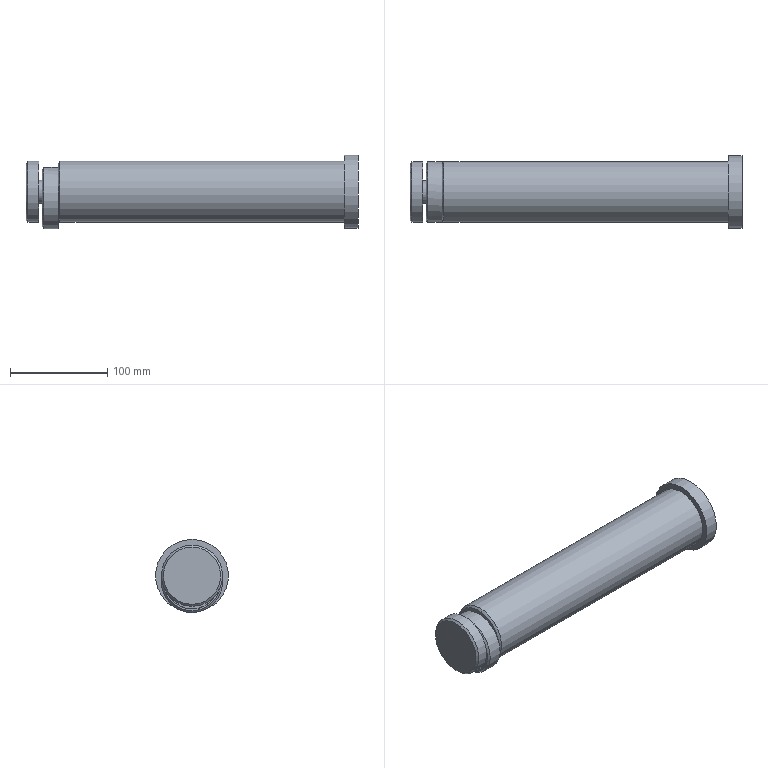Part | NX | features solid 2 | 1 solid | 17 faces | box 342 x 75 x 75.5 mm | volume 1041620 mm3 | plane 8 | cylinder 6 | cone 3 | commonest cylinder face diameters 63 x3 23.625 x1 55.5 x1 75 x1
STEP:
#1=CARTESIAN_POINT('',(940.,-806.145,-408.865));
#2=VERTEX_POINT('',#1);
#3=CARTESIAN_POINT('',(940.,-863.855,-408.865));
#4=VERTEX_POINT('',#3);
#5=CARTESIAN_POINT('',(940.,-835.,-421.5));
#6=DIRECTION('',(1.,0.,0.));
#7=DIRECTION('',(0.,0.,-1.));
#8=AXIS2_PLACEMENT_3D('',#5,#6,#7);
#9=CIRCLE('',#8,31.5);
#10=EDGE_CURVE('',#2,#4,#9,.T.);
#11=ORIENTED_EDGE('',*,*,#10,.T.);
#12=CARTESIAN_POINT('',(940.,-835.,-415.));
#13=DIRECTION('',(1.,0.,0.));
#14=DIRECTION('',(0.,0.,-1.));
#15=AXIS2_PLACEMENT_3D('',#12,#13,#14);
#16=CIRCLE('',#15,29.5);
#17=EDGE_CURVE('',#2,#4,#16,.T.);
#18=ORIENTED_EDGE('',*,*,#17,.F.);
#19=EDGE_LOOP('',(#11,#18));
#20=FACE_BOUND('',#19,.T.);
#21=CARTESIAN_POINT('',(940.,-835.,-415.));
#22=DIRECTION('',(-1.,0.,0.));
#23=DIRECTION('',(0.,0.,1.));
#24=AXIS2_PLACEMENT_3D('',#21,#22,#23);
#25=PLANE('',#24);
#26=ADVANCED_FACE('',(#20),#25,.T.);
#27=CARTESIAN_POINT('',(942.,-835.,-446.5));
#28=VERTEX_POINT('',#27);
#29=CARTESIAN_POINT('',(942.,-835.,-415.));
#30=DIRECTION('',(-1.,0.,0.));
#31=DIRECTION('',(0.,0.,-1.));
#32=AXIS2_PLACEMENT_3D('',#29,#30,#31);
#33=CIRCLE('',#32,31.5);
#34=EDGE_CURVE('',#28,#28,#33,.T.);
#35=ORIENTED_EDGE('',*,*,#34,.F.);
#36=EDGE_LOOP('',(#35));
#37=FACE_BOUND('',#36,.T.);
#38=CARTESIAN_POINT('',(1235.,-835.,-446.5));
#39=VERTEX_POINT('',#38);
#40=CARTESIAN_POINT('',(1235.,-835.,-415.));
#41=DIRECTION('',(-1.,0.,0.));
#42=DIRECTION('',(0.,0.,-1.));
#43=AXIS2_PLACEMENT_3D('',#40,#41,#42);
#44=CIRCLE('',#43,31.5);
#45=EDGE_CURVE('',#39,#39,#44,.T.);
#46=ORIENTED_EDGE('',*,*,#45,.T.);
#47=EDGE_LOOP('',(#46));
#48=FACE_BOUND('',#47,.T.);
#49=CARTESIAN_POINT('',(1235.,-835.,-415.));
#50=DIRECTION('',(-1.,0.,0.));
#51=DIRECTION('',(0.,0.,1.));
#52=AXIS2_PLACEMENT_3D('',#49,#50,#51);
#53=CYLINDRICAL_SURFACE('',#52,31.5);
#54=ADVANCED_FACE('',(#37,#48),#53,.T.);
#55=CARTESIAN_POINT('',(1249.,-835.,-377.5));
#56=VERTEX_POINT('',#55);
#57=CARTESIAN_POINT('',(1249.,-835.,-415.));
#58=DIRECTION('',(-1.,0.,0.));
#59=DIRECTION('',(0.,0.,1.));
#60=AXIS2_PLACEMENT_3D('',#57,#58,#59);
#61=CIRCLE('',#60,37.5);
#62=EDGE_CURVE('',#56,#56,#61,.T.);
#63=ORIENTED_EDGE('',*,*,#62,.F.);
#64=EDGE_LOOP('',(#63));
#65=FACE_BOUND('',#64,.T.);
#66=CARTESIAN_POINT('',(1249.,-835.,-415.));
#67=DIRECTION('',(1.,0.,0.));
#68=DIRECTION('',(0.,0.,-1.));
#69=AXIS2_PLACEMENT_3D('',#66,#67,#68);
#70=PLANE('',#69);
#71=ADVANCED_FACE('',(#65),#70,.T.);
#72=ORIENTED_EDGE('',*,*,#45,.F.);
#73=EDGE_LOOP('',(#72));
#74=FACE_BOUND('',#73,.T.);
#75=CARTESIAN_POINT('',(1235.,-835.,-377.5));
#76=VERTEX_POINT('',#75);
#77=CARTESIAN_POINT('',(1235.,-835.,-415.));
#78=DIRECTION('',(-1.,0.,0.));
#79=DIRECTION('',(0.,0.,1.));
#80=AXIS2_PLACEMENT_3D('',#77,#78,#79);
#81=CIRCLE('',#80,37.5);
#82=EDGE_CURVE('',#76,#76,#81,.T.);
#83=ORIENTED_EDGE('',*,*,#82,.T.);
#84=EDGE_LOOP('',(#83));
#85=FACE_BOUND('',#84,.T.);
#86=CARTESIAN_POINT('',(1235.,-835.,-415.));
#87=DIRECTION('',(-1.,0.,0.));
#88=DIRECTION('',(0.,0.,1.));
#89=AXIS2_PLACEMENT_3D('',#86,#87,#88);
#90=PLANE('',#89);
#91=ADVANCED_FACE('',(#74,#85),#90,.T.);
#92=ORIENTED_EDGE('',*,*,#62,.T.);
#93=EDGE_LOOP('',(#92));
#94=FACE_BOUND('',#93,.T.);
#95=ORIENTED_EDGE('',*,*,#82,.F.);
#96=EDGE_LOOP('',(#95));
#97=FACE_BOUND('',#96,.T.);
#98=CARTESIAN_POINT('',(1235.,-835.,-415.));
#99=DIRECTION('',(1.,0.,0.));
#100=DIRECTION('',(0.,0.,-1.));
#101=AXIS2_PLACEMENT_3D('',#98,#99,#100);
#102=CYLINDRICAL_SURFACE('',#101,37.5);
#103=ADVANCED_FACE('',(#94,#97),#102,.T.);
#104=ORIENTED_EDGE('',*,*,#17,.T.);
#105=CARTESIAN_POINT('',(940.,-862.39,-425.957));
#106=VERTEX_POINT('',#105);
#107=CARTESIAN_POINT('',(940.,-835.,-415.));
#108=DIRECTION('',(1.,0.,0.));
#109=DIRECTION('',(0.,0.,-1.));
#110=AXIS2_PLACEMENT_3D('',#107,#108,#109);
#111=CIRCLE('',#110,29.5);
#112=EDGE_CURVE('',#4,#106,#111,.T.);
#113=ORIENTED_EDGE('',*,*,#112,.T.);
#114=CARTESIAN_POINT('',(940.,-807.61,-425.957));
#115=VERTEX_POINT('',#114);
#116=CARTESIAN_POINT('',(940.,-835.,-415.));
#117=DIRECTION('',(1.,0.,0.));
#118=DIRECTION('',(0.,0.,-1.));
#119=AXIS2_PLACEMENT_3D('',#116,#117,#118);
#120=CIRCLE('',#119,29.5);
#121=EDGE_CURVE('',#106,#115,#120,.T.);
#122=ORIENTED_EDGE('',*,*,#121,.T.);
#123=CARTESIAN_POINT('',(940.,-835.,-415.));
#124=DIRECTION('',(1.,0.,0.));
#125=DIRECTION('',(0.,0.,-1.));
#126=AXIS2_PLACEMENT_3D('',#123,#124,#125);
#127=CIRCLE('',#126,29.5);
#128=EDGE_CURVE('',#115,#2,#127,.T.);
#129=ORIENTED_EDGE('',*,*,#128,.T.);
#130=EDGE_LOOP('',(#104,#113,#122,#129));
#131=FACE_BOUND('',#130,.T.);
#132=ORIENTED_EDGE('',*,*,#34,.T.);
#133=EDGE_LOOP('',(#132));
#134=FACE_BOUND('',#133,.T.);
#135=CARTESIAN_POINT('',(942.,-835.,-415.));
#136=DIRECTION('',(1.,0.,0.));
#137=DIRECTION('',(0.,0.,-1.));
#138=AXIS2_PLACEMENT_3D('',#135,#136,#137);
#139=CONICAL_SURFACE('',#138,31.5,0.7854);
#140=ADVANCED_FACE('',(#131,#134),#139,.T.);
#141=CARTESIAN_POINT('',(923.5,-835.,-451.));
#142=VERTEX_POINT('',#141);
#143=CARTESIAN_POINT('',(923.5,-835.,-421.5));
#144=DIRECTION('',(1.,0.,0.));
#145=DIRECTION('',(0.,0.,-1.));
#146=AXIS2_PLACEMENT_3D('',#143,#144,#145);
#147=CIRCLE('',#146,29.5);
#148=EDGE_CURVE('',#142,#142,#147,.T.);
#149=ORIENTED_EDGE('',*,*,#148,.F.);
#150=EDGE_LOOP('',(#149));
#151=FACE_BOUND('',#150,.T.);
#152=CARTESIAN_POINT('',(923.5,-835.,-393.75));
#153=VERTEX_POINT('',#152);
#154=CARTESIAN_POINT('',(923.5,-835.,-421.5));
#155=DIRECTION('',(-1.,0.,0.));
#156=DIRECTION('',(0.,0.,1.));
#157=AXIS2_PLACEMENT_3D('',#154,#155,#156);
#158=CIRCLE('',#157,27.75);
#159=EDGE_CURVE('',#153,#153,#158,.T.);
#160=ORIENTED_EDGE('',*,*,#159,.F.);
#161=EDGE_LOOP('',(#160));
#162=FACE_BOUND('',#161,.T.);
#163=CARTESIAN_POINT('',(923.5,-835.,-421.5));
#164=DIRECTION('',(-1.,0.,0.));
#165=DIRECTION('',(0.,0.,1.));
#166=AXIS2_PLACEMENT_3D('',#163,#164,#165);
#167=PLANE('',#166);
#168=ADVANCED_FACE('',(#151,#162),#167,.T.);
#169=CARTESIAN_POINT('',(940.,-835.,-421.5));
#170=DIRECTION('',(-1.,0.,0.));
#171=DIRECTION('',(0.,0.,1.));
#172=AXIS2_PLACEMENT_3D('',#169,#170,#171);
#173=CIRCLE('',#172,27.75);
#174=EDGE_CURVE('',#115,#106,#173,.T.);
#175=ORIENTED_EDGE('',*,*,#174,.T.);
#176=ORIENTED_EDGE('',*,*,#112,.F.);
#177=CARTESIAN_POINT('',(940.,-835.,-421.5));
#178=DIRECTION('',(1.,0.,0.));
#179=DIRECTION('',(0.,0.,-1.));
#180=AXIS2_PLACEMENT_3D('',#177,#178,#179);
#181=CIRCLE('',#180,31.5);
#182=EDGE_CURVE('',#4,#2,#181,.T.);
#183=ORIENTED_EDGE('',*,*,#182,.T.);
#184=ORIENTED_EDGE('',*,*,#128,.F.);
#185=EDGE_LOOP('',(#175,#176,#183,#184));
#186=FACE_BOUND('',#185,.T.);
#187=CARTESIAN_POINT('',(940.,-835.,-421.5));
#188=DIRECTION('',(1.,0.,0.));
#189=DIRECTION('',(0.,0.,-1.));
#190=AXIS2_PLACEMENT_3D('',#187,#188,#189);
#191=PLANE('',#190);
#192=ADVANCED_FACE('',(#186),#191,.T.);
#193=CARTESIAN_POINT('',(925.5,-835.,-453.));
#194=VERTEX_POINT('',#193);
#195=CARTESIAN_POINT('',(925.5,-835.,-421.5));
#196=DIRECTION('',(-1.,0.,0.));
#197=DIRECTION('',(0.,0.,-1.));
#198=AXIS2_PLACEMENT_3D('',#195,#196,#197);
#199=CIRCLE('',#198,31.5);
#200=EDGE_CURVE('',#194,#194,#199,.T.);
#201=ORIENTED_EDGE('',*,*,#200,.F.);
#202=EDGE_LOOP('',(#201));
#203=FACE_BOUND('',#202,.T.);
#204=ORIENTED_EDGE('',*,*,#10,.F.);
#205=ORIENTED_EDGE('',*,*,#182,.F.);
#206=EDGE_LOOP('',(#204,#205));
#207=FACE_BOUND('',#206,.T.);
#208=CARTESIAN_POINT('',(940.,-835.,-421.5));
#209=DIRECTION('',(-1.,0.,0.));
#210=DIRECTION('',(0.,0.,1.));
#211=AXIS2_PLACEMENT_3D('',#208,#209,#210);
#212=CYLINDRICAL_SURFACE('',#211,31.5);
#213=ADVANCED_FACE('',(#203,#207),#212,.T.);
#214=CARTESIAN_POINT('',(940.,-835.,-426.812));
#215=VERTEX_POINT('',#214);
#216=CARTESIAN_POINT('',(940.,-835.,-415.));
#217=DIRECTION('',(1.,0.,0.));
#218=DIRECTION('',(0.,0.,-1.));
#219=AXIS2_PLACEMENT_3D('',#216,#217,#218);
#220=CIRCLE('',#219,11.812);
#221=EDGE_CURVE('',#215,#215,#220,.T.);
#222=ORIENTED_EDGE('',*,*,#221,.T.);
#223=EDGE_LOOP('',(#222));
#224=FACE_BOUND('',#223,.T.);
#225=ORIENTED_EDGE('',*,*,#121,.F.);
#226=CARTESIAN_POINT('',(940.,-835.,-421.5));
#227=DIRECTION('',(-1.,0.,0.));
#228=DIRECTION('',(0.,0.,1.));
#229=AXIS2_PLACEMENT_3D('',#226,#227,#228);
#230=CIRCLE('',#229,27.75);
#231=EDGE_CURVE('',#106,#115,#230,.T.);
#232=ORIENTED_EDGE('',*,*,#231,.T.);
#233=EDGE_LOOP('',(#225,#232));
#234=FACE_BOUND('',#233,.T.);
#235=CARTESIAN_POINT('',(940.,-835.,-421.5));
#236=DIRECTION('',(1.,0.,0.));
#237=DIRECTION('',(0.,0.,-1.));
#238=AXIS2_PLACEMENT_3D('',#235,#236,#237);
#239=PLANE('',#238);
#240=ADVANCED_FACE('',(#224,#234),#239,.F.);
#241=ORIENTED_EDGE('',*,*,#174,.F.);
#242=ORIENTED_EDGE('',*,*,#231,.F.);
#243=EDGE_LOOP('',(#241,#242));
#244=FACE_BOUND('',#243,.T.);
#245=ORIENTED_EDGE('',*,*,#159,.T.);
#246=EDGE_LOOP('',(#245));
#247=FACE_BOUND('',#246,.T.);
#248=CARTESIAN_POINT('',(923.5,-835.,-421.5));
#249=DIRECTION('',(1.,0.,0.));
#250=DIRECTION('',(0.,0.,-1.));
#251=AXIS2_PLACEMENT_3D('',#248,#249,#250);
#252=CYLINDRICAL_SURFACE('',#251,27.75);
#253=ADVANCED_FACE('',(#244,#247),#252,.F.);
#254=ORIENTED_EDGE('',*,*,#200,.T.);
#255=EDGE_LOOP('',(#254));
#256=FACE_BOUND('',#255,.T.);
#257=ORIENTED_EDGE('',*,*,#148,.T.);
#258=EDGE_LOOP('',(#257));
#259=FACE_BOUND('',#258,.T.);
#260=CARTESIAN_POINT('',(923.5,-835.,-421.5));
#261=DIRECTION('',(1.,0.,0.));
#262=DIRECTION('',(0.,0.,-1.));
#263=AXIS2_PLACEMENT_3D('',#260,#261,#262);
#264=CONICAL_SURFACE('',#263,29.5,0.7854);
#265=ADVANCED_FACE('',(#256,#259),#264,.T.);
#266=CARTESIAN_POINT('',(920.2,-835.,-426.812));
#267=VERTEX_POINT('',#266);
#268=CARTESIAN_POINT('',(920.2,-835.,-415.));
#269=DIRECTION('',(1.,0.,0.));
#270=DIRECTION('',(0.,0.,-1.));
#271=AXIS2_PLACEMENT_3D('',#268,#269,#270);
#272=CIRCLE('',#271,11.812);
#273=EDGE_CURVE('',#267,#267,#272,.T.);
#274=ORIENTED_EDGE('',*,*,#273,.T.);
#275=EDGE_LOOP('',(#274));
#276=FACE_BOUND('',#275,.T.);
#277=ORIENTED_EDGE('',*,*,#221,.F.);
#278=EDGE_LOOP('',(#277));
#279=FACE_BOUND('',#278,.T.);
#280=CARTESIAN_POINT('',(940.,-835.,-415.));
#281=DIRECTION('',(-1.,0.,0.));
#282=DIRECTION('',(0.,0.,1.));
#283=AXIS2_PLACEMENT_3D('',#280,#281,#282);
#284=CYLINDRICAL_SURFACE('',#283,11.812);
#285=ADVANCED_FACE('',(#276,#279),#284,.T.);
#286=ORIENTED_EDGE('',*,*,#273,.F.);
#287=EDGE_LOOP('',(#286));
#288=FACE_BOUND('',#287,.T.);
#289=CARTESIAN_POINT('',(920.2,-835.,-383.5));
#290=VERTEX_POINT('',#289);
#291=CARTESIAN_POINT('',(920.2,-835.,-415.));
#292=DIRECTION('',(1.,0.,0.));
#293=DIRECTION('',(0.,0.,1.));
#294=AXIS2_PLACEMENT_3D('',#291,#292,#293);
#295=CIRCLE('',#294,31.5);
#296=EDGE_CURVE('',#290,#290,#295,.T.);
#297=ORIENTED_EDGE('',*,*,#296,.T.);
#298=EDGE_LOOP('',(#297));
#299=FACE_BOUND('',#298,.T.);
#300=CARTESIAN_POINT('',(920.2,-835.,-415.));
#301=DIRECTION('',(1.,0.,0.));
#302=DIRECTION('',(0.,0.,-1.));
#303=AXIS2_PLACEMENT_3D('',#300,#301,#302);
#304=PLANE('',#303);
#305=ADVANCED_FACE('',(#288,#299),#304,.T.);
#306=CARTESIAN_POINT('',(909.,-835.,-446.5));
#307=VERTEX_POINT('',#306);
#308=CARTESIAN_POINT('',(909.,-835.,-415.));
#309=DIRECTION('',(-1.,0.,0.));
#310=DIRECTION('',(0.,0.,-1.));
#311=AXIS2_PLACEMENT_3D('',#308,#309,#310);
#312=CIRCLE('',#311,31.5);
#313=EDGE_CURVE('',#307,#307,#312,.T.);
#314=ORIENTED_EDGE('',*,*,#313,.F.);
#315=EDGE_LOOP('',(#314));
#316=FACE_BOUND('',#315,.T.);
#317=ORIENTED_EDGE('',*,*,#296,.F.);
#318=EDGE_LOOP('',(#317));
#319=FACE_BOUND('',#318,.T.);
#320=CARTESIAN_POINT('',(907.,-835.,-415.));
#321=DIRECTION('',(1.,0.,0.));
#322=DIRECTION('',(0.,0.,-1.));
#323=AXIS2_PLACEMENT_3D('',#320,#321,#322);
#324=CYLINDRICAL_SURFACE('',#323,31.5);
#325=ADVANCED_FACE('',(#316,#319),#324,.T.);
#326=CARTESIAN_POINT('',(907.,-835.,-444.5));
#327=VERTEX_POINT('',#326);
#328=CARTESIAN_POINT('',(907.,-835.,-415.));
#329=DIRECTION('',(1.,0.,0.));
#330=DIRECTION('',(0.,0.,-1.));
#331=AXIS2_PLACEMENT_3D('',#328,#329,#330);
#332=CIRCLE('',#331,29.5);
#333=EDGE_CURVE('',#327,#327,#332,.T.);
#334=ORIENTED_EDGE('',*,*,#333,.F.);
#335=EDGE_LOOP('',(#334));
#336=FACE_BOUND('',#335,.T.);
#337=CARTESIAN_POINT('',(907.,-835.,-415.));
#338=DIRECTION('',(-1.,0.,0.));
#339=DIRECTION('',(0.,0.,1.));
#340=AXIS2_PLACEMENT_3D('',#337,#338,#339);
#341=PLANE('',#340);
#342=ADVANCED_FACE('',(#336),#341,.T.);
#343=ORIENTED_EDGE('',*,*,#313,.T.);
#344=EDGE_LOOP('',(#343));
#345=FACE_BOUND('',#344,.T.);
#346=ORIENTED_EDGE('',*,*,#333,.T.);
#347=EDGE_LOOP('',(#346));
#348=FACE_BOUND('',#347,.T.);
#349=CARTESIAN_POINT('',(907.,-835.,-415.));
#350=DIRECTION('',(1.,0.,0.));
#351=DIRECTION('',(0.,0.,-1.));
#352=AXIS2_PLACEMENT_3D('',#349,#350,#351);
#353=CONICAL_SURFACE('',#352,29.5,0.7854);
#354=ADVANCED_FACE('',(#345,#348),#353,.T.);
#355=CLOSED_SHELL('',(#26,#54,#71,#91,#103,#140,#168,#192,#213,#240,#253,#265,#285,#305,#325,#342,#354));
#356=MANIFOLD_SOLID_BREP('',#355);
#357=(LENGTH_UNIT()NAMED_UNIT(*)SI_UNIT(.MILLI.,.METRE.));
#358=UNCERTAINTY_MEASURE_WITH_UNIT(LENGTH_MEASURE(0.00001),#357,'','');
#359=(NAMED_UNIT(*)PLANE_ANGLE_UNIT()SI_UNIT($,.RADIAN.));
#360=(NAMED_UNIT(*)SI_UNIT($,.STERADIAN.)SOLID_ANGLE_UNIT());
#361=(GEOMETRIC_REPRESENTATION_CONTEXT(3)GLOBAL_UNCERTAINTY_ASSIGNED_CONTEXT((#358))GLOBAL_UNIT_ASSIGNED_CONTEXT((#357,#359,#360))REPRESENTATION_CONTEXT('',''));
#362=ADVANCED_BREP_SHAPE_REPRESENTATION('',(#356),#361);